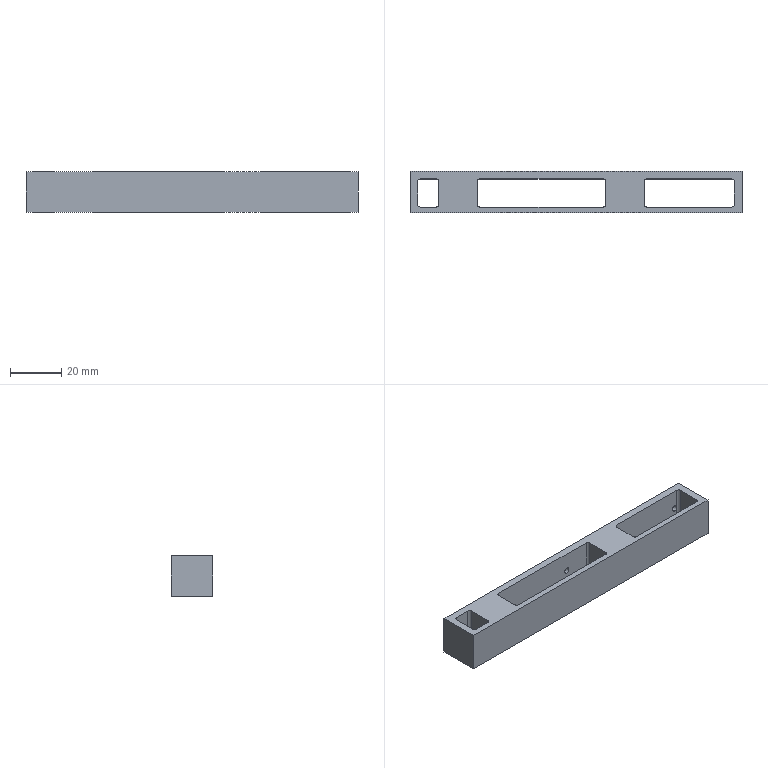Part | 1 solid | 36 faces | box 130 x 16.2 x 16 mm | volume 17152 mm3 | plane 18 | cylinder 18 | commonest cylinder face diameters 2 x12 2.4 x6
STEP:
#1=CARTESIAN_POINT('',(-65.,-8.1,-16.));
#2=VERTEX_POINT('',#1);
#3=CARTESIAN_POINT('',(65.,-8.1,-16.));
#4=VERTEX_POINT('',#3);
#5=CARTESIAN_POINT('',(-65.,-8.1,-16.));
#6=DIRECTION('',(1.,0.,0.));
#7=VECTOR('',#6,1000.);
#8=LINE('',#5,#7);
#9=EDGE_CURVE('',#2,#4,#8,.T.);
#10=ORIENTED_EDGE('',*,*,#9,.T.);
#11=CARTESIAN_POINT('',(65.,-8.1,0.));
#12=VERTEX_POINT('',#11);
#13=CARTESIAN_POINT('',(65.,-8.1,-16.));
#14=DIRECTION('',(0.,0.,1.));
#15=VECTOR('',#14,1000.);
#16=LINE('',#13,#15);
#17=EDGE_CURVE('',#4,#12,#16,.T.);
#18=ORIENTED_EDGE('',*,*,#17,.T.);
#19=CARTESIAN_POINT('',(-65.,-8.1,0.));
#20=VERTEX_POINT('',#19);
#21=CARTESIAN_POINT('',(65.,-8.1,0.));
#22=DIRECTION('',(-1.,0.,0.));
#23=VECTOR('',#22,1000.);
#24=LINE('',#21,#23);
#25=EDGE_CURVE('',#12,#20,#24,.T.);
#26=ORIENTED_EDGE('',*,*,#25,.T.);
#27=CARTESIAN_POINT('',(-65.,-8.1,-16.));
#28=DIRECTION('',(0.,0.,1.));
#29=VECTOR('',#28,1000.);
#30=LINE('',#27,#29);
#31=EDGE_CURVE('',#2,#20,#30,.T.);
#32=ORIENTED_EDGE('',*,*,#31,.F.);
#33=EDGE_LOOP('',(#10,#18,#26,#32));
#34=FACE_BOUND('',#33,.T.);
#35=CARTESIAN_POINT('',(0.,-8.1,-13.456));
#36=DIRECTION('',(0.,1.,0.));
#37=DIRECTION('',(0.,0.,-1.));
#38=AXIS2_PLACEMENT_3D('',#35,#36,#37);
#39=PLANE('',#38);
#40=ADVANCED_FACE('',(#34),#39,.F.);
#41=ORIENTED_EDGE('',*,*,#31,.T.);
#42=CARTESIAN_POINT('',(-65.,8.1,0.));
#43=VERTEX_POINT('',#42);
#44=CARTESIAN_POINT('',(-65.,-8.1,0.));
#45=DIRECTION('',(0.,1.,0.));
#46=VECTOR('',#45,1000.);
#47=LINE('',#44,#46);
#48=EDGE_CURVE('',#20,#43,#47,.T.);
#49=ORIENTED_EDGE('',*,*,#48,.T.);
#50=CARTESIAN_POINT('',(-65.,8.1,-16.));
#51=VERTEX_POINT('',#50);
#52=CARTESIAN_POINT('',(-65.,8.1,0.));
#53=DIRECTION('',(0.,0.,-1.));
#54=VECTOR('',#53,1000.);
#55=LINE('',#52,#54);
#56=EDGE_CURVE('',#43,#51,#55,.T.);
#57=ORIENTED_EDGE('',*,*,#56,.T.);
#58=CARTESIAN_POINT('',(-65.,8.1,-16.));
#59=DIRECTION('',(0.,-1.,0.));
#60=VECTOR('',#59,1000.);
#61=LINE('',#58,#60);
#62=EDGE_CURVE('',#51,#2,#61,.T.);
#63=ORIENTED_EDGE('',*,*,#62,.T.);
#64=EDGE_LOOP('',(#41,#49,#57,#63));
#65=FACE_BOUND('',#64,.T.);
#66=CARTESIAN_POINT('',(-65.,-23.95,-13.456));
#67=DIRECTION('',(1.,0.,0.));
#68=DIRECTION('',(0.,1.,0.));
#69=AXIS2_PLACEMENT_3D('',#66,#67,#68);
#70=PLANE('',#69);
#71=ADVANCED_FACE('',(#65),#70,.F.);
#72=CARTESIAN_POINT('',(65.,8.1,-16.));
#73=VERTEX_POINT('',#72);
#74=CARTESIAN_POINT('',(-65.,8.1,-16.));
#75=DIRECTION('',(1.,0.,0.));
#76=VECTOR('',#75,1000.);
#77=LINE('',#74,#76);
#78=EDGE_CURVE('',#51,#73,#77,.T.);
#79=ORIENTED_EDGE('',*,*,#78,.T.);
#80=CARTESIAN_POINT('',(65.,-8.1,-16.));
#81=DIRECTION('',(0.,1.,0.));
#82=VECTOR('',#81,1000.);
#83=LINE('',#80,#82);
#84=EDGE_CURVE('',#4,#73,#83,.T.);
#85=ORIENTED_EDGE('',*,*,#84,.F.);
#86=ORIENTED_EDGE('',*,*,#9,.F.);
#87=ORIENTED_EDGE('',*,*,#62,.F.);
#88=EDGE_LOOP('',(#79,#85,#86,#87));
#89=FACE_BOUND('',#88,.T.);
#90=CARTESIAN_POINT('',(27.702,5.1,-16.));
#91=VERTEX_POINT('',#90);
#92=CARTESIAN_POINT('',(26.702,4.1,-16.));
#93=VERTEX_POINT('',#92);
#94=CARTESIAN_POINT('',(27.702,4.1,-16.));
#95=DIRECTION('',(0.,0.,1.));
#96=DIRECTION('',(0.,1.,0.));
#97=AXIS2_PLACEMENT_3D('',#94,#95,#96);
#98=CIRCLE('',#97,1.);
#99=EDGE_CURVE('',#91,#93,#98,.T.);
#100=ORIENTED_EDGE('',*,*,#99,.T.);
#101=CARTESIAN_POINT('',(26.702,-4.9,-16.));
#102=VERTEX_POINT('',#101);
#103=CARTESIAN_POINT('',(26.702,4.1,-16.));
#104=DIRECTION('',(0.,-1.,0.));
#105=VECTOR('',#104,1000.);
#106=LINE('',#103,#105);
#107=EDGE_CURVE('',#93,#102,#106,.T.);
#108=ORIENTED_EDGE('',*,*,#107,.T.);
#109=CARTESIAN_POINT('',(27.702,-5.9,-16.));
#110=VERTEX_POINT('',#109);
#111=CARTESIAN_POINT('',(27.702,-4.9,-16.));
#112=DIRECTION('',(0.,0.,1.));
#113=DIRECTION('',(-1.,0.,0.));
#114=AXIS2_PLACEMENT_3D('',#111,#112,#113);
#115=CIRCLE('',#114,1.);
#116=EDGE_CURVE('',#102,#110,#115,.T.);
#117=ORIENTED_EDGE('',*,*,#116,.T.);
#118=CARTESIAN_POINT('',(61.,-5.9,-16.));
#119=VERTEX_POINT('',#118);
#120=CARTESIAN_POINT('',(27.702,-5.9,-16.));
#121=DIRECTION('',(1.,0.,0.));
#122=VECTOR('',#121,1000.);
#123=LINE('',#120,#122);
#124=EDGE_CURVE('',#110,#119,#123,.T.);
#125=ORIENTED_EDGE('',*,*,#124,.T.);
#126=CARTESIAN_POINT('',(62.,-4.9,-16.));
#127=VERTEX_POINT('',#126);
#128=CARTESIAN_POINT('',(61.,-4.9,-16.));
#129=DIRECTION('',(0.,0.,1.));
#130=DIRECTION('',(0.,-1.,0.));
#131=AXIS2_PLACEMENT_3D('',#128,#129,#130);
#132=CIRCLE('',#131,1.);
#133=EDGE_CURVE('',#119,#127,#132,.T.);
#134=ORIENTED_EDGE('',*,*,#133,.T.);
#135=CARTESIAN_POINT('',(62.,4.1,-16.));
#136=VERTEX_POINT('',#135);
#137=CARTESIAN_POINT('',(62.,-4.9,-16.));
#138=DIRECTION('',(0.,1.,0.));
#139=VECTOR('',#138,1000.);
#140=LINE('',#137,#139);
#141=EDGE_CURVE('',#127,#136,#140,.T.);
#142=ORIENTED_EDGE('',*,*,#141,.T.);
#143=CARTESIAN_POINT('',(61.,5.1,-16.));
#144=VERTEX_POINT('',#143);
#145=CARTESIAN_POINT('',(61.,4.1,-16.));
#146=DIRECTION('',(0.,0.,1.));
#147=DIRECTION('',(1.,0.,0.));
#148=AXIS2_PLACEMENT_3D('',#145,#146,#147);
#149=CIRCLE('',#148,1.);
#150=EDGE_CURVE('',#136,#144,#149,.T.);
#151=ORIENTED_EDGE('',*,*,#150,.T.);
#152=CARTESIAN_POINT('',(61.,5.1,-16.));
#153=DIRECTION('',(-1.,0.,0.));
#154=VECTOR('',#153,1000.);
#155=LINE('',#152,#154);
#156=EDGE_CURVE('',#144,#91,#155,.T.);
#157=ORIENTED_EDGE('',*,*,#156,.T.);
#158=EDGE_LOOP('',(#100,#108,#117,#125,#134,#142,#151,#157));
#159=FACE_BOUND('',#158,.T.);
#160=CARTESIAN_POINT('',(11.702,4.1,-16.));
#161=VERTEX_POINT('',#160);
#162=CARTESIAN_POINT('',(10.702,5.1,-16.));
#163=VERTEX_POINT('',#162);
#164=CARTESIAN_POINT('',(10.702,4.1,-16.));
#165=DIRECTION('',(0.,0.,1.));
#166=DIRECTION('',(1.,0.,0.));
#167=AXIS2_PLACEMENT_3D('',#164,#165,#166);
#168=CIRCLE('',#167,1.);
#169=EDGE_CURVE('',#161,#163,#168,.T.);
#170=ORIENTED_EDGE('',*,*,#169,.T.);
#171=CARTESIAN_POINT('',(-37.708,5.1,-16.));
#172=VERTEX_POINT('',#171);
#173=CARTESIAN_POINT('',(10.702,5.1,-16.));
#174=DIRECTION('',(-1.,0.,0.));
#175=VECTOR('',#174,1000.);
#176=LINE('',#173,#175);
#177=EDGE_CURVE('',#163,#172,#176,.T.);
#178=ORIENTED_EDGE('',*,*,#177,.T.);
#179=CARTESIAN_POINT('',(-38.708,4.1,-16.));
#180=VERTEX_POINT('',#179);
#181=CARTESIAN_POINT('',(-37.708,4.1,-16.));
#182=DIRECTION('',(0.,0.,1.));
#183=DIRECTION('',(0.,1.,0.));
#184=AXIS2_PLACEMENT_3D('',#181,#182,#183);
#185=CIRCLE('',#184,1.);
#186=EDGE_CURVE('',#172,#180,#185,.T.);
#187=ORIENTED_EDGE('',*,*,#186,.T.);
#188=CARTESIAN_POINT('',(-38.708,-4.9,-16.));
#189=VERTEX_POINT('',#188);
#190=CARTESIAN_POINT('',(-38.708,4.1,-16.));
#191=DIRECTION('',(0.,-1.,0.));
#192=VECTOR('',#191,1000.);
#193=LINE('',#190,#192);
#194=EDGE_CURVE('',#180,#189,#193,.T.);
#195=ORIENTED_EDGE('',*,*,#194,.T.);
#196=CARTESIAN_POINT('',(-37.708,-5.9,-16.));
#197=VERTEX_POINT('',#196);
#198=CARTESIAN_POINT('',(-37.708,-4.9,-16.));
#199=DIRECTION('',(0.,0.,1.));
#200=DIRECTION('',(-1.,0.,0.));
#201=AXIS2_PLACEMENT_3D('',#198,#199,#200);
#202=CIRCLE('',#201,1.);
#203=EDGE_CURVE('',#189,#197,#202,.T.);
#204=ORIENTED_EDGE('',*,*,#203,.T.);
#205=CARTESIAN_POINT('',(10.702,-5.9,-16.));
#206=VERTEX_POINT('',#205);
#207=CARTESIAN_POINT('',(-37.708,-5.9,-16.));
#208=DIRECTION('',(1.,0.,0.));
#209=VECTOR('',#208,1000.);
#210=LINE('',#207,#209);
#211=EDGE_CURVE('',#197,#206,#210,.T.);
#212=ORIENTED_EDGE('',*,*,#211,.T.);
#213=CARTESIAN_POINT('',(11.702,-4.9,-16.));
#214=VERTEX_POINT('',#213);
#215=CARTESIAN_POINT('',(10.702,-4.9,-16.));
#216=DIRECTION('',(0.,0.,1.));
#217=DIRECTION('',(0.,-1.,0.));
#218=AXIS2_PLACEMENT_3D('',#215,#216,#217);
#219=CIRCLE('',#218,1.);
#220=EDGE_CURVE('',#206,#214,#219,.T.);
#221=ORIENTED_EDGE('',*,*,#220,.T.);
#222=CARTESIAN_POINT('',(11.702,-4.9,-16.));
#223=DIRECTION('',(0.,1.,0.));
#224=VECTOR('',#223,1000.);
#225=LINE('',#222,#224);
#226=EDGE_CURVE('',#214,#161,#225,.T.);
#227=ORIENTED_EDGE('',*,*,#226,.T.);
#228=EDGE_LOOP('',(#170,#178,#187,#195,#204,#212,#221,#227));
#229=FACE_BOUND('',#228,.T.);
#230=CARTESIAN_POINT('',(-61.,5.1,-16.));
#231=VERTEX_POINT('',#230);
#232=CARTESIAN_POINT('',(-62.,4.1,-16.));
#233=VERTEX_POINT('',#232);
#234=CARTESIAN_POINT('',(-61.,4.1,-16.));
#235=DIRECTION('',(0.,0.,1.));
#236=DIRECTION('',(0.,1.,0.));
#237=AXIS2_PLACEMENT_3D('',#234,#235,#236);
#238=CIRCLE('',#237,1.);
#239=EDGE_CURVE('',#231,#233,#238,.T.);
#240=ORIENTED_EDGE('',*,*,#239,.T.);
#241=CARTESIAN_POINT('',(-62.,-4.9,-16.));
#242=VERTEX_POINT('',#241);
#243=CARTESIAN_POINT('',(-62.,4.1,-16.));
#244=DIRECTION('',(0.,-1.,0.));
#245=VECTOR('',#244,1000.);
#246=LINE('',#243,#245);
#247=EDGE_CURVE('',#233,#242,#246,.T.);
#248=ORIENTED_EDGE('',*,*,#247,.T.);
#249=CARTESIAN_POINT('',(-61.,-5.9,-16.));
#250=VERTEX_POINT('',#249);
#251=CARTESIAN_POINT('',(-61.,-4.9,-16.));
#252=DIRECTION('',(0.,0.,1.));
#253=DIRECTION('',(-1.,0.,0.));
#254=AXIS2_PLACEMENT_3D('',#251,#252,#253);
#255=CIRCLE('',#254,1.);
#256=EDGE_CURVE('',#242,#250,#255,.T.);
#257=ORIENTED_EDGE('',*,*,#256,.T.);
#258=CARTESIAN_POINT('',(-54.708,-5.9,-16.));
#259=VERTEX_POINT('',#258);
#260=CARTESIAN_POINT('',(-61.,-5.9,-16.));
#261=DIRECTION('',(1.,0.,0.));
#262=VECTOR('',#261,1000.);
#263=LINE('',#260,#262);
#264=EDGE_CURVE('',#250,#259,#263,.T.);
#265=ORIENTED_EDGE('',*,*,#264,.T.);
#266=CARTESIAN_POINT('',(-53.708,-4.9,-16.));
#267=VERTEX_POINT('',#266);
#268=CARTESIAN_POINT('',(-54.708,-4.9,-16.));
#269=DIRECTION('',(0.,0.,1.));
#270=DIRECTION('',(0.,-1.,0.));
#271=AXIS2_PLACEMENT_3D('',#268,#269,#270);
#272=CIRCLE('',#271,1.);
#273=EDGE_CURVE('',#259,#267,#272,.T.);
#274=ORIENTED_EDGE('',*,*,#273,.T.);
#275=CARTESIAN_POINT('',(-53.708,4.1,-16.));
#276=VERTEX_POINT('',#275);
#277=CARTESIAN_POINT('',(-53.708,-4.9,-16.));
#278=DIRECTION('',(0.,1.,0.));
#279=VECTOR('',#278,1000.);
#280=LINE('',#277,#279);
#281=EDGE_CURVE('',#267,#276,#280,.T.);
#282=ORIENTED_EDGE('',*,*,#281,.T.);
#283=CARTESIAN_POINT('',(-54.708,5.1,-16.));
#284=VERTEX_POINT('',#283);
#285=CARTESIAN_POINT('',(-54.708,4.1,-16.));
#286=DIRECTION('',(0.,0.,1.));
#287=DIRECTION('',(1.,0.,0.));
#288=AXIS2_PLACEMENT_3D('',#285,#286,#287);
#289=CIRCLE('',#288,1.);
#290=EDGE_CURVE('',#276,#284,#289,.T.);
#291=ORIENTED_EDGE('',*,*,#290,.T.);
#292=CARTESIAN_POINT('',(-54.708,5.1,-16.));
#293=DIRECTION('',(-1.,0.,0.));
#294=VECTOR('',#293,1000.);
#295=LINE('',#292,#294);
#296=EDGE_CURVE('',#284,#231,#295,.T.);
#297=ORIENTED_EDGE('',*,*,#296,.T.);
#298=EDGE_LOOP('',(#240,#248,#257,#265,#274,#282,#291,#297));
#299=FACE_BOUND('',#298,.T.);
#300=CARTESIAN_POINT('',(-65.,-8.9,-16.));
#301=DIRECTION('',(0.,0.,-1.));
#302=DIRECTION('',(0.,-1.,0.));
#303=AXIS2_PLACEMENT_3D('',#300,#301,#302);
#304=PLANE('',#303);
#305=ADVANCED_FACE('',(#89,#159,#229,#299),#304,.T.);
#306=CARTESIAN_POINT('',(65.,8.1,0.));
#307=VERTEX_POINT('',#306);
#308=CARTESIAN_POINT('',(65.,8.1,-16.));
#309=DIRECTION('',(0.,0.,1.));
#310=VECTOR('',#309,1000.);
#311=LINE('',#308,#310);
#312=EDGE_CURVE('',#73,#307,#311,.T.);
#313=ORIENTED_EDGE('',*,*,#312,.T.);
#314=CARTESIAN_POINT('',(65.,8.1,0.));
#315=DIRECTION('',(0.,-1.,0.));
#316=VECTOR('',#315,1000.);
#317=LINE('',#314,#316);
#318=EDGE_CURVE('',#307,#12,#317,.T.);
#319=ORIENTED_EDGE('',*,*,#318,.T.);
#320=ORIENTED_EDGE('',*,*,#17,.F.);
#321=ORIENTED_EDGE('',*,*,#84,.T.);
#322=EDGE_LOOP('',(#313,#319,#320,#321));
#323=FACE_BOUND('',#322,.T.);
#324=CARTESIAN_POINT('',(65.,-23.95,-13.456));
#325=DIRECTION('',(1.,0.,0.));
#326=DIRECTION('',(0.,1.,0.));
#327=AXIS2_PLACEMENT_3D('',#324,#325,#326);
#328=PLANE('',#327);
#329=ADVANCED_FACE('',(#323),#328,.T.);
#330=ORIENTED_EDGE('',*,*,#25,.F.);
#331=ORIENTED_EDGE('',*,*,#318,.F.);
#332=CARTESIAN_POINT('',(-65.,8.1,0.));
#333=DIRECTION('',(1.,0.,0.));
#334=VECTOR('',#333,1000.);
#335=LINE('',#332,#334);
#336=EDGE_CURVE('',#43,#307,#335,.T.);
#337=ORIENTED_EDGE('',*,*,#336,.F.);
#338=ORIENTED_EDGE('',*,*,#48,.F.);
#339=EDGE_LOOP('',(#330,#331,#337,#338));
#340=FACE_BOUND('',#339,.T.);
#341=CARTESIAN_POINT('',(62.,-4.9,0.));
#342=VERTEX_POINT('',#341);
#343=CARTESIAN_POINT('',(61.,-5.9,0.));
#344=VERTEX_POINT('',#343);
#345=CARTESIAN_POINT('',(61.,-4.9,0.));
#346=DIRECTION('',(0.,0.,-1.));
#347=DIRECTION('',(1.,0.,0.));
#348=AXIS2_PLACEMENT_3D('',#345,#346,#347);
#349=CIRCLE('',#348,1.);
#350=EDGE_CURVE('',#342,#344,#349,.T.);
#351=ORIENTED_EDGE('',*,*,#350,.T.);
#352=CARTESIAN_POINT('',(27.702,-5.9,0.));
#353=VERTEX_POINT('',#352);
#354=CARTESIAN_POINT('',(27.702,-5.9,0.));
#355=DIRECTION('',(1.,0.,0.));
#356=VECTOR('',#355,1000.);
#357=LINE('',#354,#356);
#358=EDGE_CURVE('',#353,#344,#357,.T.);
#359=ORIENTED_EDGE('',*,*,#358,.F.);
#360=CARTESIAN_POINT('',(26.702,-4.9,0.));
#361=VERTEX_POINT('',#360);
#362=CARTESIAN_POINT('',(27.702,-4.9,0.));
#363=DIRECTION('',(0.,0.,-1.));
#364=DIRECTION('',(0.,-1.,0.));
#365=AXIS2_PLACEMENT_3D('',#362,#363,#364);
#366=CIRCLE('',#365,1.);
#367=EDGE_CURVE('',#353,#361,#366,.T.);
#368=ORIENTED_EDGE('',*,*,#367,.T.);
#369=CARTESIAN_POINT('',(26.702,4.1,0.));
#370=VERTEX_POINT('',#369);
#371=CARTESIAN_POINT('',(26.702,4.1,0.));
#372=DIRECTION('',(0.,-1.,0.));
#373=VECTOR('',#372,1000.);
#374=LINE('',#371,#373);
#375=EDGE_CURVE('',#370,#361,#374,.T.);
#376=ORIENTED_EDGE('',*,*,#375,.F.);
#377=CARTESIAN_POINT('',(27.702,5.1,0.));
#378=VERTEX_POINT('',#377);
#379=CARTESIAN_POINT('',(27.702,4.1,0.));
#380=DIRECTION('',(0.,0.,-1.));
#381=DIRECTION('',(-1.,0.,0.));
#382=AXIS2_PLACEMENT_3D('',#379,#380,#381);
#383=CIRCLE('',#382,1.);
#384=EDGE_CURVE('',#370,#378,#383,.T.);
#385=ORIENTED_EDGE('',*,*,#384,.T.);
#386=CARTESIAN_POINT('',(61.,5.1,0.));
#387=VERTEX_POINT('',#386);
#388=CARTESIAN_POINT('',(61.,5.1,0.));
#389=DIRECTION('',(-1.,0.,0.));
#390=VECTOR('',#389,1000.);
#391=LINE('',#388,#390);
#392=EDGE_CURVE('',#387,#378,#391,.T.);
#393=ORIENTED_EDGE('',*,*,#392,.F.);
#394=CARTESIAN_POINT('',(62.,4.1,0.));
#395=VERTEX_POINT('',#394);
#396=CARTESIAN_POINT('',(61.,4.1,0.));
#397=DIRECTION('',(0.,0.,-1.));
#398=DIRECTION('',(0.,1.,0.));
#399=AXIS2_PLACEMENT_3D('',#396,#397,#398);
#400=CIRCLE('',#399,1.);
#401=EDGE_CURVE('',#387,#395,#400,.T.);
#402=ORIENTED_EDGE('',*,*,#401,.T.);
#403=CARTESIAN_POINT('',(62.,-4.9,0.));
#404=DIRECTION('',(0.,1.,0.));
#405=VECTOR('',#404,1000.);
#406=LINE('',#403,#405);
#407=EDGE_CURVE('',#342,#395,#406,.T.);
#408=ORIENTED_EDGE('',*,*,#407,.F.);
#409=EDGE_LOOP('',(#351,#359,#368,#376,#385,#393,#402,#408));
#410=FACE_BOUND('',#409,.T.);
#411=CARTESIAN_POINT('',(-37.708,-5.9,0.));
#412=VERTEX_POINT('',#411);
#413=CARTESIAN_POINT('',(-38.708,-4.9,0.));
#414=VERTEX_POINT('',#413);
#415=CARTESIAN_POINT('',(-37.708,-4.9,0.));
#416=DIRECTION('',(0.,0.,-1.));
#417=DIRECTION('',(0.,-1.,0.));
#418=AXIS2_PLACEMENT_3D('',#415,#416,#417);
#419=CIRCLE('',#418,1.);
#420=EDGE_CURVE('',#412,#414,#419,.T.);
#421=ORIENTED_EDGE('',*,*,#420,.T.);
#422=CARTESIAN_POINT('',(-38.708,4.1,0.));
#423=VERTEX_POINT('',#422);
#424=CARTESIAN_POINT('',(-38.708,4.1,0.));
#425=DIRECTION('',(0.,-1.,0.));
#426=VECTOR('',#425,1000.);
#427=LINE('',#424,#426);
#428=EDGE_CURVE('',#423,#414,#427,.T.);
#429=ORIENTED_EDGE('',*,*,#428,.F.);
#430=CARTESIAN_POINT('',(-37.708,5.1,0.));
#431=VERTEX_POINT('',#430);
#432=CARTESIAN_POINT('',(-37.708,4.1,0.));
#433=DIRECTION('',(0.,0.,-1.));
#434=DIRECTION('',(-1.,0.,0.));
#435=AXIS2_PLACEMENT_3D('',#432,#433,#434);
#436=CIRCLE('',#435,1.);
#437=EDGE_CURVE('',#423,#431,#436,.T.);
#438=ORIENTED_EDGE('',*,*,#437,.T.);
#439=CARTESIAN_POINT('',(10.702,5.1,0.));
#440=VERTEX_POINT('',#439);
#441=CARTESIAN_POINT('',(10.702,5.1,0.));
#442=DIRECTION('',(-1.,0.,0.));
#443=VECTOR('',#442,1000.);
#444=LINE('',#441,#443);
#445=EDGE_CURVE('',#440,#431,#444,.T.);
#446=ORIENTED_EDGE('',*,*,#445,.F.);
#447=CARTESIAN_POINT('',(11.702,4.1,0.));
#448=VERTEX_POINT('',#447);
#449=CARTESIAN_POINT('',(10.702,4.1,0.));
#450=DIRECTION('',(0.,0.,-1.));
#451=DIRECTION('',(0.,1.,0.));
#452=AXIS2_PLACEMENT_3D('',#449,#450,#451);
#453=CIRCLE('',#452,1.);
#454=EDGE_CURVE('',#440,#448,#453,.T.);
#455=ORIENTED_EDGE('',*,*,#454,.T.);
#456=CARTESIAN_POINT('',(11.702,-4.9,0.));
#457=VERTEX_POINT('',#456);
#458=CARTESIAN_POINT('',(11.702,-4.9,0.));
#459=DIRECTION('',(0.,1.,0.));
#460=VECTOR('',#459,1000.);
#461=LINE('',#458,#460);
#462=EDGE_CURVE('',#457,#448,#461,.T.);
#463=ORIENTED_EDGE('',*,*,#462,.F.);
#464=CARTESIAN_POINT('',(10.702,-5.9,0.));
#465=VERTEX_POINT('',#464);
#466=CARTESIAN_POINT('',(10.702,-4.9,0.));
#467=DIRECTION('',(0.,0.,-1.));
#468=DIRECTION('',(1.,0.,0.));
#469=AXIS2_PLACEMENT_3D('',#466,#467,#468);
#470=CIRCLE('',#469,1.);
#471=EDGE_CURVE('',#457,#465,#470,.T.);
#472=ORIENTED_EDGE('',*,*,#471,.T.);
#473=CARTESIAN_POINT('',(-37.708,-5.9,0.));
#474=DIRECTION('',(1.,0.,0.));
#475=VECTOR('',#474,1000.);
#476=LINE('',#473,#475);
#477=EDGE_CURVE('',#412,#465,#476,.T.);
#478=ORIENTED_EDGE('',*,*,#477,.F.);
#479=EDGE_LOOP('',(#421,#429,#438,#446,#455,#463,#472,#478));
#480=FACE_BOUND('',#479,.T.);
#481=CARTESIAN_POINT('',(-53.708,-4.9,0.));
#482=VERTEX_POINT('',#481);
#483=CARTESIAN_POINT('',(-54.708,-5.9,0.));
#484=VERTEX_POINT('',#483);
#485=CARTESIAN_POINT('',(-54.708,-4.9,0.));
#486=DIRECTION('',(0.,0.,-1.));
#487=DIRECTION('',(1.,0.,0.));
#488=AXIS2_PLACEMENT_3D('',#485,#486,#487);
#489=CIRCLE('',#488,1.);
#490=EDGE_CURVE('',#482,#484,#489,.T.);
#491=ORIENTED_EDGE('',*,*,#490,.T.);
#492=CARTESIAN_POINT('',(-61.,-5.9,0.));
#493=VERTEX_POINT('',#492);
#494=CARTESIAN_POINT('',(-61.,-5.9,0.));
#495=DIRECTION('',(1.,0.,0.));
#496=VECTOR('',#495,1000.);
#497=LINE('',#494,#496);
#498=EDGE_CURVE('',#493,#484,#497,.T.);
#499=ORIENTED_EDGE('',*,*,#498,.F.);
#500=CARTESIAN_POINT('',(-62.,-4.9,0.));
#501=VERTEX_POINT('',#500);
#502=CARTESIAN_POINT('',(-61.,-4.9,0.));
#503=DIRECTION('',(0.,0.,-1.));
#504=DIRECTION('',(0.,-1.,0.));
#505=AXIS2_PLACEMENT_3D('',#502,#503,#504);
#506=CIRCLE('',#505,1.);
#507=EDGE_CURVE('',#493,#501,#506,.T.);
#508=ORIENTED_EDGE('',*,*,#507,.T.);
#509=CARTESIAN_POINT('',(-62.,4.1,0.));
#510=VERTEX_POINT('',#509);
#511=CARTESIAN_POINT('',(-62.,-4.9,0.));
#512=DIRECTION('',(0.,1.,0.));
#513=VECTOR('',#512,1000.);
#514=LINE('',#511,#513);
#515=EDGE_CURVE('',#501,#510,#514,.T.);
#516=ORIENTED_EDGE('',*,*,#515,.T.);
#517=CARTESIAN_POINT('',(-61.,5.1,0.));
#518=VERTEX_POINT('',#517);
#519=CARTESIAN_POINT('',(-61.,4.1,0.));
#520=DIRECTION('',(0.,0.,-1.));
#521=DIRECTION('',(-1.,0.,0.));
#522=AXIS2_PLACEMENT_3D('',#519,#520,#521);
#523=CIRCLE('',#522,1.);
#524=EDGE_CURVE('',#510,#518,#523,.T.);
#525=ORIENTED_EDGE('',*,*,#524,.T.);
#526=CARTESIAN_POINT('',(-54.708,5.1,0.));
#527=VERTEX_POINT('',#526);
#528=CARTESIAN_POINT('',(-54.708,5.1,0.));
#529=DIRECTION('',(-1.,0.,0.));
#530=VECTOR('',#529,1000.);
#531=LINE('',#528,#530);
#532=EDGE_CURVE('',#527,#518,#531,.T.);
#533=ORIENTED_EDGE('',*,*,#532,.F.);
#534=CARTESIAN_POINT('',(-53.708,4.1,0.));
#535=VERTEX_POINT('',#534);
#536=CARTESIAN_POINT('',(-54.708,4.1,0.));
#537=DIRECTION('',(0.,0.,-1.));
#538=DIRECTION('',(0.,1.,0.));
#539=AXIS2_PLACEMENT_3D('',#536,#537,#538);
#540=CIRCLE('',#539,1.);
#541=EDGE_CURVE('',#527,#535,#540,.T.);
#542=ORIENTED_EDGE('',*,*,#541,.T.);
#543=CARTESIAN_POINT('',(-53.708,-4.9,0.));
#544=DIRECTION('',(0.,1.,0.));
#545=VECTOR('',#544,1000.);
#546=LINE('',#543,#545);
#547=EDGE_CURVE('',#482,#535,#546,.T.);
#548=ORIENTED_EDGE('',*,*,#547,.F.);
#549=EDGE_LOOP('',(#491,#499,#508,#516,#525,#533,#542,#548));
#550=FACE_BOUND('',#549,.T.);
#551=CARTESIAN_POINT('',(-50.708,-9.1,0.));
#552=DIRECTION('',(0.,0.,1.));
#553=DIRECTION('',(-1.,0.,0.));
#554=AXIS2_PLACEMENT_3D('',#551,#552,#553);
#555=PLANE('',#554);
#556=ADVANCED_FACE('',(#340,#410,#480,#550),#555,.T.);
#557=ORIENTED_EDGE('',*,*,#56,.F.);
#558=ORIENTED_EDGE('',*,*,#336,.T.);
#559=ORIENTED_EDGE('',*,*,#312,.F.);
#560=ORIENTED_EDGE('',*,*,#78,.F.);
#561=EDGE_LOOP('',(#557,#558,#559,#560));
#562=FACE_BOUND('',#561,.T.);
#563=CARTESIAN_POINT('',(-59.8,8.1,-6.8));
#564=VERTEX_POINT('',#563);
#565=CARTESIAN_POINT('',(-59.8,8.1,-9.2));
#566=VERTEX_POINT('',#565);
#567=CARTESIAN_POINT('',(-59.8,8.1,-8.));
#568=DIRECTION('',(0.,1.,0.));
#569=DIRECTION('',(0.,0.,1.));
#570=AXIS2_PLACEMENT_3D('',#567,#568,#569);
#571=CIRCLE('',#570,1.2);
#572=EDGE_CURVE('',#564,#566,#571,.T.);
#573=ORIENTED_EDGE('',*,*,#572,.F.);
#574=CARTESIAN_POINT('',(-59.8,8.1,-8.));
#575=DIRECTION('',(0.,1.,0.));
#576=DIRECTION('',(0.,0.,-1.));
#577=AXIS2_PLACEMENT_3D('',#574,#575,#576);
#578=CIRCLE('',#577,1.2);
#579=EDGE_CURVE('',#566,#564,#578,.T.);
#580=ORIENTED_EDGE('',*,*,#579,.F.);
#581=EDGE_LOOP('',(#573,#580));
#582=FACE_BOUND('',#581,.T.);
#583=CARTESIAN_POINT('',(59.8,8.1,-6.8));
#584=VERTEX_POINT('',#583);
#585=CARTESIAN_POINT('',(59.8,8.1,-9.2));
#586=VERTEX_POINT('',#585);
#587=CARTESIAN_POINT('',(59.8,8.1,-8.));
#588=DIRECTION('',(0.,1.,0.));
#589=DIRECTION('',(0.,0.,1.));
#590=AXIS2_PLACEMENT_3D('',#587,#588,#589);
#591=CIRCLE('',#590,1.2);
#592=EDGE_CURVE('',#584,#586,#591,.T.);
#593=ORIENTED_EDGE('',*,*,#592,.F.);
#594=CARTESIAN_POINT('',(59.8,8.1,-8.));
#595=DIRECTION('',(0.,1.,0.));
#596=DIRECTION('',(0.,0.,-1.));
#597=AXIS2_PLACEMENT_3D('',#594,#595,#596);
#598=CIRCLE('',#597,1.2);
#599=EDGE_CURVE('',#586,#584,#598,.T.);
#600=ORIENTED_EDGE('',*,*,#599,.F.);
#601=EDGE_LOOP('',(#593,#600));
#602=FACE_BOUND('',#601,.T.);
#603=CARTESIAN_POINT('',(0.,8.1,-6.8));
#604=VERTEX_POINT('',#603);
#605=CARTESIAN_POINT('',(0.,8.1,-9.2));
#606=VERTEX_POINT('',#605);
#607=CARTESIAN_POINT('',(0.,8.1,-8.));
#608=DIRECTION('',(0.,1.,0.));
#609=DIRECTION('',(0.,0.,1.));
#610=AXIS2_PLACEMENT_3D('',#607,#608,#609);
#611=CIRCLE('',#610,1.2);
#612=EDGE_CURVE('',#604,#606,#611,.T.);
#613=ORIENTED_EDGE('',*,*,#612,.F.);
#614=CARTESIAN_POINT('',(0.,8.1,-8.));
#615=DIRECTION('',(0.,1.,0.));
#616=DIRECTION('',(0.,0.,-1.));
#617=AXIS2_PLACEMENT_3D('',#614,#615,#616);
#618=CIRCLE('',#617,1.2);
#619=EDGE_CURVE('',#606,#604,#618,.T.);
#620=ORIENTED_EDGE('',*,*,#619,.F.);
#621=EDGE_LOOP('',(#613,#620));
#622=FACE_BOUND('',#621,.T.);
#623=CARTESIAN_POINT('',(-65.,8.1,-32.913));
#624=DIRECTION('',(0.,1.,0.));
#625=DIRECTION('',(0.,0.,-1.));
#626=AXIS2_PLACEMENT_3D('',#623,#624,#625);
#627=PLANE('',#626);
#628=ADVANCED_FACE('',(#562,#582,#602,#622),#627,.T.);
#629=CARTESIAN_POINT('',(-59.8,5.1,-6.8));
#630=VERTEX_POINT('',#629);
#631=CARTESIAN_POINT('',(-59.8,8.1,-6.8));
#632=DIRECTION('',(0.,-1.,0.));
#633=VECTOR('',#632,1000.);
#634=LINE('',#631,#633);
#635=EDGE_CURVE('',#564,#630,#634,.T.);
#636=ORIENTED_EDGE('',*,*,#635,.T.);
#637=CARTESIAN_POINT('',(-61.,5.1,-8.));
#638=VERTEX_POINT('',#637);
#639=CARTESIAN_POINT('',(-59.8,5.1,-8.));
#640=DIRECTION('',(0.,1.,0.));
#641=DIRECTION('',(-1.,0.,0.));
#642=AXIS2_PLACEMENT_3D('',#639,#640,#641);
#643=CIRCLE('',#642,1.2);
#644=EDGE_CURVE('',#638,#630,#643,.T.);
#645=ORIENTED_EDGE('',*,*,#644,.F.);
#646=CARTESIAN_POINT('',(-59.8,5.1,-9.2));
#647=VERTEX_POINT('',#646);
#648=CARTESIAN_POINT('',(-59.8,5.1,-8.));
#649=DIRECTION('',(0.,1.,0.));
#650=DIRECTION('',(0.,0.,-1.));
#651=AXIS2_PLACEMENT_3D('',#648,#649,#650);
#652=CIRCLE('',#651,1.2);
#653=EDGE_CURVE('',#647,#638,#652,.T.);
#654=ORIENTED_EDGE('',*,*,#653,.F.);
#655=CARTESIAN_POINT('',(-59.8,8.1,-9.2));
#656=DIRECTION('',(0.,-1.,0.));
#657=VECTOR('',#656,1000.);
#658=LINE('',#655,#657);
#659=EDGE_CURVE('',#566,#647,#658,.T.);
#660=ORIENTED_EDGE('',*,*,#659,.F.);
#661=ORIENTED_EDGE('',*,*,#579,.T.);
#662=EDGE_LOOP('',(#636,#645,#654,#660,#661));
#663=FACE_BOUND('',#662,.T.);
#664=CARTESIAN_POINT('',(-59.8,8.1,-8.));
#665=DIRECTION('',(0.,1.,0.));
#666=DIRECTION('',(0.,0.,1.));
#667=AXIS2_PLACEMENT_3D('',#664,#665,#666);
#668=CYLINDRICAL_SURFACE('',#667,1.2);
#669=ADVANCED_FACE('',(#663),#668,.F.);
#670=ORIENTED_EDGE('',*,*,#659,.T.);
#671=CARTESIAN_POINT('',(-59.8,5.1,-8.));
#672=DIRECTION('',(0.,1.,0.));
#673=DIRECTION('',(0.,0.,1.));
#674=AXIS2_PLACEMENT_3D('',#671,#672,#673);
#675=CIRCLE('',#674,1.2);
#676=EDGE_CURVE('',#630,#647,#675,.T.);
#677=ORIENTED_EDGE('',*,*,#676,.F.);
#678=ORIENTED_EDGE('',*,*,#635,.F.);
#679=ORIENTED_EDGE('',*,*,#572,.T.);
#680=EDGE_LOOP('',(#670,#677,#678,#679));
#681=FACE_BOUND('',#680,.T.);
#682=CARTESIAN_POINT('',(-59.8,8.1,-8.));
#683=DIRECTION('',(0.,1.,0.));
#684=DIRECTION('',(0.,0.,1.));
#685=AXIS2_PLACEMENT_3D('',#682,#683,#684);
#686=CYLINDRICAL_SURFACE('',#685,1.2);
#687=ADVANCED_FACE('',(#681),#686,.F.);
#688=CARTESIAN_POINT('',(-61.,5.1,-16.));
#689=DIRECTION('',(0.,0.,1.));
#690=VECTOR('',#689,1000.);
#691=LINE('',#688,#690);
#692=EDGE_CURVE('',#231,#638,#691,.T.);
#693=ORIENTED_EDGE('',*,*,#692,.F.);
#694=ORIENTED_EDGE('',*,*,#296,.F.);
#695=CARTESIAN_POINT('',(-54.708,5.1,0.));
#696=DIRECTION('',(0.,0.,-1.));
#697=VECTOR('',#696,1000.);
#698=LINE('',#695,#697);
#699=EDGE_CURVE('',#527,#284,#698,.T.);
#700=ORIENTED_EDGE('',*,*,#699,.F.);
#701=ORIENTED_EDGE('',*,*,#532,.T.);
#702=CARTESIAN_POINT('',(-61.,5.1,-8.));
#703=DIRECTION('',(0.,0.,1.));
#704=VECTOR('',#703,1000.);
#705=LINE('',#702,#704);
#706=EDGE_CURVE('',#638,#518,#705,.T.);
#707=ORIENTED_EDGE('',*,*,#706,.F.);
#708=ORIENTED_EDGE('',*,*,#644,.T.);
#709=ORIENTED_EDGE('',*,*,#676,.T.);
#710=ORIENTED_EDGE('',*,*,#653,.T.);
#711=EDGE_LOOP('',(#693,#694,#700,#701,#707,#708,#709,#710));
#712=FACE_BOUND('',#711,.T.);
#713=CARTESIAN_POINT('',(-53.708,5.1,0.));
#714=DIRECTION('',(0.,1.,0.));
#715=DIRECTION('',(1.,0.,0.));
#716=AXIS2_PLACEMENT_3D('',#713,#714,#715);
#717=PLANE('',#716);
#718=ADVANCED_FACE('',(#712),#717,.F.);
#719=ORIENTED_EDGE('',*,*,#706,.T.);
#720=ORIENTED_EDGE('',*,*,#524,.F.);
#721=CARTESIAN_POINT('',(-62.,4.1,-16.));
#722=DIRECTION('',(0.,0.,1.));
#723=VECTOR('',#722,1000.);
#724=LINE('',#721,#723);
#725=EDGE_CURVE('',#233,#510,#724,.T.);
#726=ORIENTED_EDGE('',*,*,#725,.F.);
#727=ORIENTED_EDGE('',*,*,#239,.F.);
#728=ORIENTED_EDGE('',*,*,#692,.T.);
#729=EDGE_LOOP('',(#719,#720,#726,#727,#728));
#730=FACE_BOUND('',#729,.T.);
#731=CARTESIAN_POINT('',(-61.,4.1,-273.236));
#732=DIRECTION('',(0.,0.,1.));
#733=DIRECTION('',(0.,-1.,0.));
#734=AXIS2_PLACEMENT_3D('',#731,#732,#733);
#735=CYLINDRICAL_SURFACE('',#734,1.);
#736=ADVANCED_FACE('',(#730),#735,.F.);
#737=ORIENTED_EDGE('',*,*,#247,.F.);
#738=ORIENTED_EDGE('',*,*,#725,.T.);
#739=ORIENTED_EDGE('',*,*,#515,.F.);
#740=CARTESIAN_POINT('',(-62.,-4.9,0.));
#741=DIRECTION('',(0.,0.,-1.));
#742=VECTOR('',#741,1000.);
#743=LINE('',#740,#742);
#744=EDGE_CURVE('',#501,#242,#743,.T.);
#745=ORIENTED_EDGE('',*,*,#744,.T.);
#746=EDGE_LOOP('',(#737,#738,#739,#745));
#747=FACE_BOUND('',#746,.T.);
#748=CARTESIAN_POINT('',(-62.,-23.95,-13.456));
#749=DIRECTION('',(-1.,0.,0.));
#750=DIRECTION('',(0.,0.,-1.));
#751=AXIS2_PLACEMENT_3D('',#748,#749,#750);
#752=PLANE('',#751);
#753=ADVANCED_FACE('',(#747),#752,.F.);
#754=ORIENTED_EDGE('',*,*,#256,.F.);
#755=ORIENTED_EDGE('',*,*,#744,.F.);
#756=ORIENTED_EDGE('',*,*,#507,.F.);
#757=CARTESIAN_POINT('',(-61.,-5.9,0.));
#758=DIRECTION('',(0.,0.,-1.));
#759=VECTOR('',#758,1000.);
#760=LINE('',#757,#759);
#761=EDGE_CURVE('',#493,#250,#760,.T.);
#762=ORIENTED_EDGE('',*,*,#761,.T.);
#763=EDGE_LOOP('',(#754,#755,#756,#762));
#764=FACE_BOUND('',#763,.T.);
#765=CARTESIAN_POINT('',(-61.,-4.9,258.925));
#766=DIRECTION('',(0.,0.,-1.));
#767=DIRECTION('',(0.,1.,0.));
#768=AXIS2_PLACEMENT_3D('',#765,#766,#767);
#769=CYLINDRICAL_SURFACE('',#768,1.);
#770=ADVANCED_FACE('',(#764),#769,.F.);
#771=ORIENTED_EDGE('',*,*,#264,.F.);
#772=ORIENTED_EDGE('',*,*,#761,.F.);
#773=ORIENTED_EDGE('',*,*,#498,.T.);
#774=CARTESIAN_POINT('',(-54.708,-5.9,0.));
#775=DIRECTION('',(0.,0.,-1.));
#776=VECTOR('',#775,1000.);
#777=LINE('',#774,#776);
#778=EDGE_CURVE('',#484,#259,#777,.T.);
#779=ORIENTED_EDGE('',*,*,#778,.T.);
#780=EDGE_LOOP('',(#771,#772,#773,#779));
#781=FACE_BOUND('',#780,.T.);
#782=CARTESIAN_POINT('',(-66.9,-5.9,0.));
#783=DIRECTION('',(0.,-1.,0.));
#784=DIRECTION('',(-1.,0.,0.));
#785=AXIS2_PLACEMENT_3D('',#782,#783,#784);
#786=PLANE('',#785);
#787=ADVANCED_FACE('',(#781),#786,.F.);
#788=ORIENTED_EDGE('',*,*,#273,.F.);
#789=ORIENTED_EDGE('',*,*,#778,.F.);
#790=ORIENTED_EDGE('',*,*,#490,.F.);
#791=CARTESIAN_POINT('',(-53.708,-4.9,0.));
#792=DIRECTION('',(0.,0.,-1.));
#793=VECTOR('',#792,1000.);
#794=LINE('',#791,#793);
#795=EDGE_CURVE('',#482,#267,#794,.T.);
#796=ORIENTED_EDGE('',*,*,#795,.T.);
#797=EDGE_LOOP('',(#788,#789,#790,#796));
#798=FACE_BOUND('',#797,.T.);
#799=CARTESIAN_POINT('',(-54.708,-4.9,242.536));
#800=DIRECTION('',(0.,0.,-1.));
#801=DIRECTION('',(-1.,0.,0.));
#802=AXIS2_PLACEMENT_3D('',#799,#800,#801);
#803=CYLINDRICAL_SURFACE('',#802,1.);
#804=ADVANCED_FACE('',(#798),#803,.F.);
#805=ORIENTED_EDGE('',*,*,#281,.F.);
#806=ORIENTED_EDGE('',*,*,#795,.F.);
#807=ORIENTED_EDGE('',*,*,#547,.T.);
#808=CARTESIAN_POINT('',(-53.708,4.1,0.));
#809=DIRECTION('',(0.,0.,-1.));
#810=VECTOR('',#809,1000.);
#811=LINE('',#808,#810);
#812=EDGE_CURVE('',#535,#276,#811,.T.);
#813=ORIENTED_EDGE('',*,*,#812,.T.);
#814=EDGE_LOOP('',(#805,#806,#807,#813));
#815=FACE_BOUND('',#814,.T.);
#816=CARTESIAN_POINT('',(-53.708,-5.9,0.));
#817=DIRECTION('',(1.,0.,0.));
#818=DIRECTION('',(0.,-1.,0.));
#819=AXIS2_PLACEMENT_3D('',#816,#817,#818);
#820=PLANE('',#819);
#821=ADVANCED_FACE('',(#815),#820,.F.);
#822=ORIENTED_EDGE('',*,*,#290,.F.);
#823=ORIENTED_EDGE('',*,*,#812,.F.);
#824=ORIENTED_EDGE('',*,*,#541,.F.);
#825=ORIENTED_EDGE('',*,*,#699,.T.);
#826=EDGE_LOOP('',(#822,#823,#824,#825));
#827=FACE_BOUND('',#826,.T.);
#828=CARTESIAN_POINT('',(-54.708,4.1,242.564));
#829=DIRECTION('',(0.,0.,-1.));
#830=DIRECTION('',(0.,-1.,0.));
#831=AXIS2_PLACEMENT_3D('',#828,#829,#830);
#832=CYLINDRICAL_SURFACE('',#831,1.);
#833=ADVANCED_FACE('',(#827),#832,.F.);
#834=CARTESIAN_POINT('',(59.8,5.1,-6.8));
#835=VERTEX_POINT('',#834);
#836=CARTESIAN_POINT('',(59.8,8.1,-6.8));
#837=DIRECTION('',(0.,-1.,0.));
#838=VECTOR('',#837,1000.);
#839=LINE('',#836,#838);
#840=EDGE_CURVE('',#584,#835,#839,.T.);
#841=ORIENTED_EDGE('',*,*,#840,.T.);
#842=CARTESIAN_POINT('',(59.8,5.1,-9.2));
#843=VERTEX_POINT('',#842);
#844=CARTESIAN_POINT('',(59.8,5.1,-8.));
#845=DIRECTION('',(0.,1.,0.));
#846=DIRECTION('',(0.,0.,-1.));
#847=AXIS2_PLACEMENT_3D('',#844,#845,#846);
#848=CIRCLE('',#847,1.2);
#849=EDGE_CURVE('',#843,#835,#848,.T.);
#850=ORIENTED_EDGE('',*,*,#849,.F.);
#851=CARTESIAN_POINT('',(59.8,8.1,-9.2));
#852=DIRECTION('',(0.,-1.,0.));
#853=VECTOR('',#852,1000.);
#854=LINE('',#851,#853);
#855=EDGE_CURVE('',#586,#843,#854,.T.);
#856=ORIENTED_EDGE('',*,*,#855,.F.);
#857=ORIENTED_EDGE('',*,*,#599,.T.);
#858=EDGE_LOOP('',(#841,#850,#856,#857));
#859=FACE_BOUND('',#858,.T.);
#860=CARTESIAN_POINT('',(59.8,8.1,-8.));
#861=DIRECTION('',(0.,1.,0.));
#862=DIRECTION('',(0.,0.,1.));
#863=AXIS2_PLACEMENT_3D('',#860,#861,#862);
#864=CYLINDRICAL_SURFACE('',#863,1.2);
#865=ADVANCED_FACE('',(#859),#864,.F.);
#866=ORIENTED_EDGE('',*,*,#855,.T.);
#867=CARTESIAN_POINT('',(61.,5.1,-8.));
#868=VERTEX_POINT('',#867);
#869=CARTESIAN_POINT('',(59.8,5.1,-8.));
#870=DIRECTION('',(0.,1.,0.));
#871=DIRECTION('',(1.,0.,0.));
#872=AXIS2_PLACEMENT_3D('',#869,#870,#871);
#873=CIRCLE('',#872,1.2);
#874=EDGE_CURVE('',#868,#843,#873,.T.);
#875=ORIENTED_EDGE('',*,*,#874,.F.);
#876=CARTESIAN_POINT('',(59.8,5.1,-8.));
#877=DIRECTION('',(0.,1.,0.));
#878=DIRECTION('',(0.,0.,1.));
#879=AXIS2_PLACEMENT_3D('',#876,#877,#878);
#880=CIRCLE('',#879,1.2);
#881=EDGE_CURVE('',#835,#868,#880,.T.);
#882=ORIENTED_EDGE('',*,*,#881,.F.);
#883=ORIENTED_EDGE('',*,*,#840,.F.);
#884=ORIENTED_EDGE('',*,*,#592,.T.);
#885=EDGE_LOOP('',(#866,#875,#882,#883,#884));
#886=FACE_BOUND('',#885,.T.);
#887=CARTESIAN_POINT('',(59.8,8.1,-8.));
#888=DIRECTION('',(0.,1.,0.));
#889=DIRECTION('',(0.,0.,1.));
#890=AXIS2_PLACEMENT_3D('',#887,#888,#889);
#891=CYLINDRICAL_SURFACE('',#890,1.2);
#892=ADVANCED_FACE('',(#886),#891,.F.);
#893=ORIENTED_EDGE('',*,*,#881,.T.);
#894=CARTESIAN_POINT('',(61.,5.1,0.));
#895=DIRECTION('',(0.,0.,-1.));
#896=VECTOR('',#895,1000.);
#897=LINE('',#894,#896);
#898=EDGE_CURVE('',#387,#868,#897,.T.);
#899=ORIENTED_EDGE('',*,*,#898,.F.);
#900=ORIENTED_EDGE('',*,*,#392,.T.);
#901=CARTESIAN_POINT('',(27.702,5.1,0.));
#902=DIRECTION('',(0.,0.,-1.));
#903=VECTOR('',#902,1000.);
#904=LINE('',#901,#903);
#905=EDGE_CURVE('',#378,#91,#904,.T.);
#906=ORIENTED_EDGE('',*,*,#905,.T.);
#907=ORIENTED_EDGE('',*,*,#156,.F.);
#908=CARTESIAN_POINT('',(61.,5.1,-8.));
#909=DIRECTION('',(0.,0.,-1.));
#910=VECTOR('',#909,1000.);
#911=LINE('',#908,#910);
#912=EDGE_CURVE('',#868,#144,#911,.T.);
#913=ORIENTED_EDGE('',*,*,#912,.F.);
#914=ORIENTED_EDGE('',*,*,#874,.T.);
#915=ORIENTED_EDGE('',*,*,#849,.T.);
#916=EDGE_LOOP('',(#893,#899,#900,#906,#907,#913,#914,#915));
#917=FACE_BOUND('',#916,.T.);
#918=CARTESIAN_POINT('',(62.,5.1,0.));
#919=DIRECTION('',(0.,1.,0.));
#920=DIRECTION('',(1.,0.,0.));
#921=AXIS2_PLACEMENT_3D('',#918,#919,#920);
#922=PLANE('',#921);
#923=ADVANCED_FACE('',(#917),#922,.F.);
#924=ORIENTED_EDGE('',*,*,#912,.T.);
#925=ORIENTED_EDGE('',*,*,#150,.F.);
#926=CARTESIAN_POINT('',(62.,4.1,0.));
#927=DIRECTION('',(0.,0.,-1.));
#928=VECTOR('',#927,1000.);
#929=LINE('',#926,#928);
#930=EDGE_CURVE('',#395,#136,#929,.T.);
#931=ORIENTED_EDGE('',*,*,#930,.F.);
#932=ORIENTED_EDGE('',*,*,#401,.F.);
#933=ORIENTED_EDGE('',*,*,#898,.T.);
#934=EDGE_LOOP('',(#924,#925,#931,#932,#933));
#935=FACE_BOUND('',#934,.T.);
#936=CARTESIAN_POINT('',(61.,4.1,258.925));
#937=DIRECTION('',(0.,0.,-1.));
#938=DIRECTION('',(0.,-1.,0.));
#939=AXIS2_PLACEMENT_3D('',#936,#937,#938);
#940=CYLINDRICAL_SURFACE('',#939,1.);
#941=ADVANCED_FACE('',(#935),#940,.F.);
#942=ORIENTED_EDGE('',*,*,#407,.T.);
#943=ORIENTED_EDGE('',*,*,#930,.T.);
#944=ORIENTED_EDGE('',*,*,#141,.F.);
#945=CARTESIAN_POINT('',(62.,-4.9,0.));
#946=DIRECTION('',(0.,0.,-1.));
#947=VECTOR('',#946,1000.);
#948=LINE('',#945,#947);
#949=EDGE_CURVE('',#342,#127,#948,.T.);
#950=ORIENTED_EDGE('',*,*,#949,.F.);
#951=EDGE_LOOP('',(#942,#943,#944,#950));
#952=FACE_BOUND('',#951,.T.);
#953=CARTESIAN_POINT('',(62.,-5.9,0.));
#954=DIRECTION('',(1.,0.,0.));
#955=DIRECTION('',(0.,-1.,0.));
#956=AXIS2_PLACEMENT_3D('',#953,#954,#955);
#957=PLANE('',#956);
#958=ADVANCED_FACE('',(#952),#957,.F.);
#959=ORIENTED_EDGE('',*,*,#133,.F.);
#960=CARTESIAN_POINT('',(61.,-5.9,0.));
#961=DIRECTION('',(0.,0.,-1.));
#962=VECTOR('',#961,1000.);
#963=LINE('',#960,#962);
#964=EDGE_CURVE('',#344,#119,#963,.T.);
#965=ORIENTED_EDGE('',*,*,#964,.F.);
#966=ORIENTED_EDGE('',*,*,#350,.F.);
#967=ORIENTED_EDGE('',*,*,#949,.T.);
#968=EDGE_LOOP('',(#959,#965,#966,#967));
#969=FACE_BOUND('',#968,.T.);
#970=CARTESIAN_POINT('',(61.,-4.9,257.477));
#971=DIRECTION('',(0.,0.,-1.));
#972=DIRECTION('',(-1.,0.,0.));
#973=AXIS2_PLACEMENT_3D('',#970,#971,#972);
#974=CYLINDRICAL_SURFACE('',#973,1.);
#975=ADVANCED_FACE('',(#969),#974,.F.);
#976=ORIENTED_EDGE('',*,*,#124,.F.);
#977=CARTESIAN_POINT('',(27.702,-5.9,0.));
#978=DIRECTION('',(0.,0.,-1.));
#979=VECTOR('',#978,1000.);
#980=LINE('',#977,#979);
#981=EDGE_CURVE('',#353,#110,#980,.T.);
#982=ORIENTED_EDGE('',*,*,#981,.F.);
#983=ORIENTED_EDGE('',*,*,#358,.T.);
#984=ORIENTED_EDGE('',*,*,#964,.T.);
#985=EDGE_LOOP('',(#976,#982,#983,#984));
#986=FACE_BOUND('',#985,.T.);
#987=CARTESIAN_POINT('',(26.702,-5.9,0.));
#988=DIRECTION('',(0.,-1.,0.));
#989=DIRECTION('',(-1.,0.,0.));
#990=AXIS2_PLACEMENT_3D('',#987,#988,#989);
#991=PLANE('',#990);
#992=ADVANCED_FACE('',(#986),#991,.F.);
#993=ORIENTED_EDGE('',*,*,#116,.F.);
#994=CARTESIAN_POINT('',(26.702,-4.9,0.));
#995=DIRECTION('',(0.,0.,-1.));
#996=VECTOR('',#995,1000.);
#997=LINE('',#994,#996);
#998=EDGE_CURVE('',#361,#102,#997,.T.);
#999=ORIENTED_EDGE('',*,*,#998,.F.);
#1000=ORIENTED_EDGE('',*,*,#367,.F.);
#1001=ORIENTED_EDGE('',*,*,#981,.T.);
#1002=EDGE_LOOP('',(#993,#999,#1000,#1001));
#1003=FACE_BOUND('',#1002,.T.);
#1004=CARTESIAN_POINT('',(27.702,-4.9,189.534));
#1005=DIRECTION('',(0.,0.,-1.));
#1006=DIRECTION('',(0.,1.,0.));
#1007=AXIS2_PLACEMENT_3D('',#1004,#1005,#1006);
#1008=CYLINDRICAL_SURFACE('',#1007,1.);
#1009=ADVANCED_FACE('',(#1003),#1008,.F.);
#1010=ORIENTED_EDGE('',*,*,#107,.F.);
#1011=CARTESIAN_POINT('',(26.702,4.1,0.));
#1012=DIRECTION('',(0.,0.,-1.));
#1013=VECTOR('',#1012,1000.);
#1014=LINE('',#1011,#1013);
#1015=EDGE_CURVE('',#370,#93,#1014,.T.);
#1016=ORIENTED_EDGE('',*,*,#1015,.F.);
#1017=ORIENTED_EDGE('',*,*,#375,.T.);
#1018=ORIENTED_EDGE('',*,*,#998,.T.);
#1019=EDGE_LOOP('',(#1010,#1016,#1017,#1018));
#1020=FACE_BOUND('',#1019,.T.);
#1021=CARTESIAN_POINT('',(26.702,5.1,0.));
#1022=DIRECTION('',(-1.,0.,0.));
#1023=DIRECTION('',(0.,1.,0.));
#1024=AXIS2_PLACEMENT_3D('',#1021,#1022,#1023);
#1025=PLANE('',#1024);
#1026=ADVANCED_FACE('',(#1020),#1025,.F.);
#1027=ORIENTED_EDGE('',*,*,#99,.F.);
#1028=ORIENTED_EDGE('',*,*,#905,.F.);
#1029=ORIENTED_EDGE('',*,*,#384,.F.);
#1030=ORIENTED_EDGE('',*,*,#1015,.T.);
#1031=EDGE_LOOP('',(#1027,#1028,#1029,#1030));
#1032=FACE_BOUND('',#1031,.T.);
#1033=CARTESIAN_POINT('',(27.702,4.1,189.452));
#1034=DIRECTION('',(0.,0.,-1.));
#1035=DIRECTION('',(1.,0.,0.));
#1036=AXIS2_PLACEMENT_3D('',#1033,#1034,#1035);
#1037=CYLINDRICAL_SURFACE('',#1036,1.);
#1038=ADVANCED_FACE('',(#1032),#1037,.F.);
#1039=CARTESIAN_POINT('',(0.,5.1,-6.8));
#1040=VERTEX_POINT('',#1039);
#1041=CARTESIAN_POINT('',(0.,8.1,-6.8));
#1042=DIRECTION('',(0.,-1.,0.));
#1043=VECTOR('',#1042,1000.);
#1044=LINE('',#1041,#1043);
#1045=EDGE_CURVE('',#604,#1040,#1044,.T.);
#1046=ORIENTED_EDGE('',*,*,#1045,.T.);
#1047=CARTESIAN_POINT('',(0.,5.1,-9.2));
#1048=VERTEX_POINT('',#1047);
#1049=CARTESIAN_POINT('',(0.,5.1,-8.));
#1050=DIRECTION('',(0.,1.,0.));
#1051=DIRECTION('',(0.,0.,-1.));
#1052=AXIS2_PLACEMENT_3D('',#1049,#1050,#1051);
#1053=CIRCLE('',#1052,1.2);
#1054=EDGE_CURVE('',#1048,#1040,#1053,.T.);
#1055=ORIENTED_EDGE('',*,*,#1054,.F.);
#1056=CARTESIAN_POINT('',(0.,8.1,-9.2));
#1057=DIRECTION('',(0.,-1.,0.));
#1058=VECTOR('',#1057,1000.);
#1059=LINE('',#1056,#1058);
#1060=EDGE_CURVE('',#606,#1048,#1059,.T.);
#1061=ORIENTED_EDGE('',*,*,#1060,.F.);
#1062=ORIENTED_EDGE('',*,*,#619,.T.);
#1063=EDGE_LOOP('',(#1046,#1055,#1061,#1062));
#1064=FACE_BOUND('',#1063,.T.);
#1065=CARTESIAN_POINT('',(0.,8.1,-8.));
#1066=DIRECTION('',(0.,1.,0.));
#1067=DIRECTION('',(0.,0.,1.));
#1068=AXIS2_PLACEMENT_3D('',#1065,#1066,#1067);
#1069=CYLINDRICAL_SURFACE('',#1068,1.2);
#1070=ADVANCED_FACE('',(#1064),#1069,.F.);
#1071=ORIENTED_EDGE('',*,*,#1060,.T.);
#1072=CARTESIAN_POINT('',(0.,5.1,-8.));
#1073=DIRECTION('',(0.,1.,0.));
#1074=DIRECTION('',(0.,0.,1.));
#1075=AXIS2_PLACEMENT_3D('',#1072,#1073,#1074);
#1076=CIRCLE('',#1075,1.2);
#1077=EDGE_CURVE('',#1040,#1048,#1076,.T.);
#1078=ORIENTED_EDGE('',*,*,#1077,.F.);
#1079=ORIENTED_EDGE('',*,*,#1045,.F.);
#1080=ORIENTED_EDGE('',*,*,#612,.T.);
#1081=EDGE_LOOP('',(#1071,#1078,#1079,#1080));
#1082=FACE_BOUND('',#1081,.T.);
#1083=CARTESIAN_POINT('',(0.,8.1,-8.));
#1084=DIRECTION('',(0.,1.,0.));
#1085=DIRECTION('',(0.,0.,1.));
#1086=AXIS2_PLACEMENT_3D('',#1083,#1084,#1085);
#1087=CYLINDRICAL_SURFACE('',#1086,1.2);
#1088=ADVANCED_FACE('',(#1082),#1087,.F.);
#1089=ORIENTED_EDGE('',*,*,#445,.T.);
#1090=CARTESIAN_POINT('',(-37.708,5.1,0.));
#1091=DIRECTION('',(0.,0.,-1.));
#1092=VECTOR('',#1091,1000.);
#1093=LINE('',#1090,#1092);
#1094=EDGE_CURVE('',#431,#172,#1093,.T.);
#1095=ORIENTED_EDGE('',*,*,#1094,.T.);
#1096=ORIENTED_EDGE('',*,*,#177,.F.);
#1097=CARTESIAN_POINT('',(10.702,5.1,0.));
#1098=DIRECTION('',(0.,0.,-1.));
#1099=VECTOR('',#1098,1000.);
#1100=LINE('',#1097,#1099);
#1101=EDGE_CURVE('',#440,#163,#1100,.T.);
#1102=ORIENTED_EDGE('',*,*,#1101,.F.);
#1103=EDGE_LOOP('',(#1089,#1095,#1096,#1102));
#1104=FACE_BOUND('',#1103,.T.);
#1105=ORIENTED_EDGE('',*,*,#1077,.T.);
#1106=ORIENTED_EDGE('',*,*,#1054,.T.);
#1107=EDGE_LOOP('',(#1105,#1106));
#1108=FACE_BOUND('',#1107,.T.);
#1109=CARTESIAN_POINT('',(11.702,5.1,0.));
#1110=DIRECTION('',(0.,1.,0.));
#1111=DIRECTION('',(1.,0.,0.));
#1112=AXIS2_PLACEMENT_3D('',#1109,#1110,#1111);
#1113=PLANE('',#1112);
#1114=ADVANCED_FACE('',(#1104,#1108),#1113,.F.);
#1115=ORIENTED_EDGE('',*,*,#169,.F.);
#1116=CARTESIAN_POINT('',(11.702,4.1,0.));
#1117=DIRECTION('',(0.,0.,-1.));
#1118=VECTOR('',#1117,1000.);
#1119=LINE('',#1116,#1118);
#1120=EDGE_CURVE('',#448,#161,#1119,.T.);
#1121=ORIENTED_EDGE('',*,*,#1120,.F.);
#1122=ORIENTED_EDGE('',*,*,#454,.F.);
#1123=ORIENTED_EDGE('',*,*,#1101,.T.);
#1124=EDGE_LOOP('',(#1115,#1121,#1122,#1123));
#1125=FACE_BOUND('',#1124,.T.);
#1126=CARTESIAN_POINT('',(10.702,4.1,160.396));
#1127=DIRECTION('',(0.,0.,-1.));
#1128=DIRECTION('',(0.,-1.,0.));
#1129=AXIS2_PLACEMENT_3D('',#1126,#1127,#1128);
#1130=CYLINDRICAL_SURFACE('',#1129,1.);
#1131=ADVANCED_FACE('',(#1125),#1130,.F.);
#1132=ORIENTED_EDGE('',*,*,#462,.T.);
#1133=ORIENTED_EDGE('',*,*,#1120,.T.);
#1134=ORIENTED_EDGE('',*,*,#226,.F.);
#1135=CARTESIAN_POINT('',(11.702,-4.9,0.));
#1136=DIRECTION('',(0.,0.,-1.));
#1137=VECTOR('',#1136,1000.);
#1138=LINE('',#1135,#1137);
#1139=EDGE_CURVE('',#457,#214,#1138,.T.);
#1140=ORIENTED_EDGE('',*,*,#1139,.F.);
#1141=EDGE_LOOP('',(#1132,#1133,#1134,#1140));
#1142=FACE_BOUND('',#1141,.T.);
#1143=CARTESIAN_POINT('',(11.702,-5.9,0.));
#1144=DIRECTION('',(1.,0.,0.));
#1145=DIRECTION('',(0.,-1.,0.));
#1146=AXIS2_PLACEMENT_3D('',#1143,#1144,#1145);
#1147=PLANE('',#1146);
#1148=ADVANCED_FACE('',(#1142),#1147,.F.);
#1149=ORIENTED_EDGE('',*,*,#220,.F.);
#1150=CARTESIAN_POINT('',(10.702,-5.9,0.));
#1151=DIRECTION('',(0.,0.,-1.));
#1152=VECTOR('',#1151,1000.);
#1153=LINE('',#1150,#1152);
#1154=EDGE_CURVE('',#465,#206,#1153,.T.);
#1155=ORIENTED_EDGE('',*,*,#1154,.F.);
#1156=ORIENTED_EDGE('',*,*,#471,.F.);
#1157=ORIENTED_EDGE('',*,*,#1139,.T.);
#1158=EDGE_LOOP('',(#1149,#1155,#1156,#1157));
#1159=FACE_BOUND('',#1158,.T.);
#1160=CARTESIAN_POINT('',(10.702,-4.9,160.285));
#1161=DIRECTION('',(0.,0.,-1.));
#1162=DIRECTION('',(-1.,0.,0.));
#1163=AXIS2_PLACEMENT_3D('',#1160,#1161,#1162);
#1164=CYLINDRICAL_SURFACE('',#1163,1.);
#1165=ADVANCED_FACE('',(#1159),#1164,.F.);
#1166=ORIENTED_EDGE('',*,*,#211,.F.);
#1167=CARTESIAN_POINT('',(-37.708,-5.9,0.));
#1168=DIRECTION('',(0.,0.,-1.));
#1169=VECTOR('',#1168,1000.);
#1170=LINE('',#1167,#1169);
#1171=EDGE_CURVE('',#412,#197,#1170,.T.);
#1172=ORIENTED_EDGE('',*,*,#1171,.F.);
#1173=ORIENTED_EDGE('',*,*,#477,.T.);
#1174=ORIENTED_EDGE('',*,*,#1154,.T.);
#1175=EDGE_LOOP('',(#1166,#1172,#1173,#1174));
#1176=FACE_BOUND('',#1175,.T.);
#1177=CARTESIAN_POINT('',(-38.708,-5.9,0.));
#1178=DIRECTION('',(0.,-1.,0.));
#1179=DIRECTION('',(-1.,0.,0.));
#1180=AXIS2_PLACEMENT_3D('',#1177,#1178,#1179);
#1181=PLANE('',#1180);
#1182=ADVANCED_FACE('',(#1176),#1181,.F.);
#1183=ORIENTED_EDGE('',*,*,#203,.F.);
#1184=CARTESIAN_POINT('',(-38.708,-4.9,0.));
#1185=DIRECTION('',(0.,0.,-1.));
#1186=VECTOR('',#1185,1000.);
#1187=LINE('',#1184,#1186);
#1188=EDGE_CURVE('',#414,#189,#1187,.T.);
#1189=ORIENTED_EDGE('',*,*,#1188,.F.);
#1190=ORIENTED_EDGE('',*,*,#420,.F.);
#1191=ORIENTED_EDGE('',*,*,#1171,.T.);
#1192=EDGE_LOOP('',(#1183,#1189,#1190,#1191));
#1193=FACE_BOUND('',#1192,.T.);
#1194=CARTESIAN_POINT('',(-37.708,-4.9,212.984));
#1195=DIRECTION('',(0.,0.,-1.));
#1196=DIRECTION('',(0.,1.,0.));
#1197=AXIS2_PLACEMENT_3D('',#1194,#1195,#1196);
#1198=CYLINDRICAL_SURFACE('',#1197,1.);
#1199=ADVANCED_FACE('',(#1193),#1198,.F.);
#1200=ORIENTED_EDGE('',*,*,#428,.T.);
#1201=ORIENTED_EDGE('',*,*,#1188,.T.);
#1202=ORIENTED_EDGE('',*,*,#194,.F.);
#1203=CARTESIAN_POINT('',(-38.708,4.1,0.));
#1204=DIRECTION('',(0.,0.,-1.));
#1205=VECTOR('',#1204,1000.);
#1206=LINE('',#1203,#1205);
#1207=EDGE_CURVE('',#423,#180,#1206,.T.);
#1208=ORIENTED_EDGE('',*,*,#1207,.F.);
#1209=EDGE_LOOP('',(#1200,#1201,#1202,#1208));
#1210=FACE_BOUND('',#1209,.T.);
#1211=CARTESIAN_POINT('',(-38.708,5.1,0.));
#1212=DIRECTION('',(-1.,0.,0.));
#1213=DIRECTION('',(0.,1.,0.));
#1214=AXIS2_PLACEMENT_3D('',#1211,#1212,#1213);
#1215=PLANE('',#1214);
#1216=ADVANCED_FACE('',(#1210),#1215,.F.);
#1217=ORIENTED_EDGE('',*,*,#186,.F.);
#1218=ORIENTED_EDGE('',*,*,#1094,.F.);
#1219=ORIENTED_EDGE('',*,*,#437,.F.);
#1220=ORIENTED_EDGE('',*,*,#1207,.T.);
#1221=EDGE_LOOP('',(#1217,#1218,#1219,#1220));
#1222=FACE_BOUND('',#1221,.T.);
#1223=CARTESIAN_POINT('',(-37.708,4.1,211.264));
#1224=DIRECTION('',(0.,0.,-1.));
#1225=DIRECTION('',(1.,0.,0.));
#1226=AXIS2_PLACEMENT_3D('',#1223,#1224,#1225);
#1227=CYLINDRICAL_SURFACE('',#1226,1.);
#1228=ADVANCED_FACE('',(#1222),#1227,.F.);
#1229=CLOSED_SHELL('',(#40,#71,#305,#329,#556,#628,#669,#687,#718,#736,#753,#770,#787,#804,#821,#833,#865,#892,#923,#941,#958,#975,#992,#1009,#1026,#1038,#1070,#1088,#1114,#1131,#1148,#1165,#1182,#1199,#1216,#1228));
#1230=MANIFOLD_SOLID_BREP('',#1229);
#1231=(LENGTH_UNIT()NAMED_UNIT(*)SI_UNIT(.MILLI.,.METRE.));
#1232=UNCERTAINTY_MEASURE_WITH_UNIT(LENGTH_MEASURE(0.00001),#1231,'','');
#1233=(NAMED_UNIT(*)PLANE_ANGLE_UNIT()SI_UNIT($,.RADIAN.));
#1234=(NAMED_UNIT(*)SI_UNIT($,.STERADIAN.)SOLID_ANGLE_UNIT());
#1235=(GEOMETRIC_REPRESENTATION_CONTEXT(3)GLOBAL_UNCERTAINTY_ASSIGNED_CONTEXT((#1232))GLOBAL_UNIT_ASSIGNED_CONTEXT((#1231,#1233,#1234))REPRESENTATION_CONTEXT('',''));
#1236=ADVANCED_BREP_SHAPE_REPRESENTATION('',(#1230),#1235);